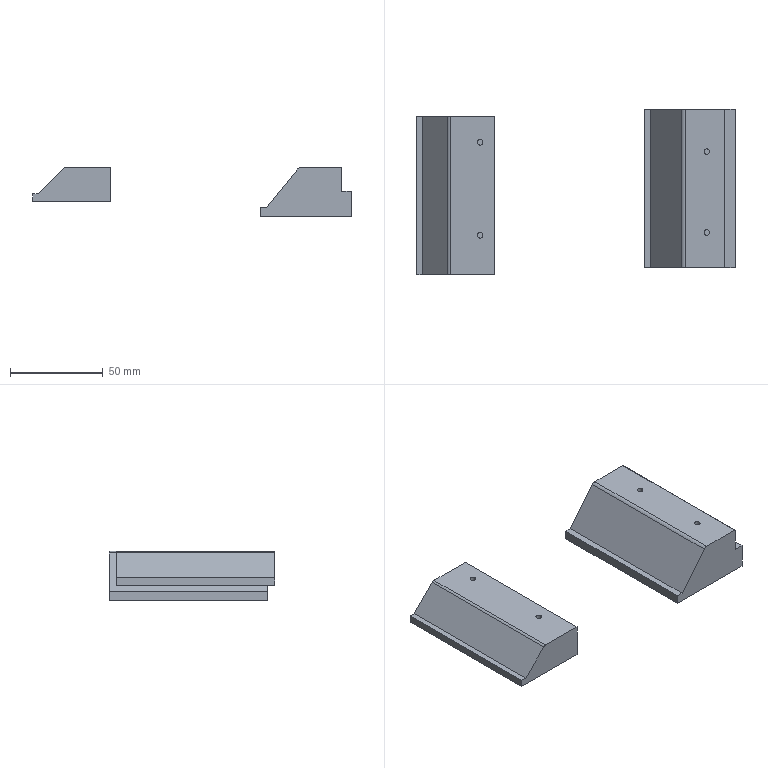NC program | NX | posted with a generic post | part box 171.319 x 88.841 x 26.598 mm
Lines 1 to 928 of 2519:
N10 G17 G21 G94 G90
(FLOOR_WALL_COPY , TOOL : D80)
N12 T19 M6
N14 G54
N16 G17 G0 G90 X91.5 Y0. S6500 M3
N18 G43 Z30. H19
N20 Z3.
N22 G94 G1 Z0. F1500.
N24 X86.5
N26 X-86.5
N28 X-91.5
N30 Z3.
N32 G0 Z30.
N34 M5
(ADAPTIVE_MILLING , TOOL : D10)
N36 T15 M6
N38 G54
N40 G17 G0 G90 X0.049 Y-32.696 S9500 M3
N42 G43 Z30. H15
N44 Z-15.302
N46 G94 G1 Z-18.302 F1000.
N48 X0.579 Y-31.339 F3000.
N50 G3 X0.049 Y-30.049 R1.015
N52 X-3.11 Y-29.406 R9.424
N54 X-14.606 Y-29.21 R185.073
N56 G1 X-20.006 Y-29.208
N58 X-43.706 Y-29.207
N60 X-43.906 Y-29.205
N62 X-44.006 Y-29.201
N64 X-44.106 Y-29.195
N66 X-44.206 Y-29.187
N68 G2 X-48.539 Y-26.275 R6.033
N70 X-50.327 Y-20.706 R13.143
N72 X-50.675 Y-12.117 R79.626
N74 G1 X-50.681 Y-10.617
N76 X-50.686 Y-8.517
N78 X-50.689 Y-4.917
N80 X-50.69 Y8.783
N82 Y22.283
N84 X-50.689 Y22.383
N86 G2 X-48.028 Y26.859 R5.823
N88 X-42.511 Y28.786 R12.484
N90 X-34.025 Y29.173 R71.151
N92 G1 X-32.625 Y29.18
N94 X-30.725 Y29.185
N96 X-27.725 Y29.188
N98 X-20.025 Y29.19
N100 X43.775
N102 X43.875 Y29.189
N104 G2 X48.354 Y26.533 R5.826
N106 X50.283 Y21.017 R12.389
N108 X50.675 Y12.031 R75.333
N110 G1 X50.682 Y10.532
N112 X50.687 Y8.332
N114 X50.689 Y4.632
N116 X50.69 Y-10.868
N118 Y-22.268
N120 Y-22.368
N122 G2 X48.201 Y-26.732 R5.739
N124 X42.821 Y-28.739 R11.862
N126 X34.639 Y-29.167 R61.998
N128 G1 X33.439 Y-29.176
N130 X31.839 Y-29.182
N132 X29.639 Y-29.187
N134 X25.639 Y-29.189
N136 X3.439 Y-29.19
N138 X3.239 Y-29.188
N140 G2 X-2.538 Y-28.69 R147.004
N142 G3 X-15.232 Y-28.421 R195.936
N144 G1 X-18.532 Y-28.418
N146 X-26.232 Y-28.416
N148 X-41.032
N150 X-41.232 Y-28.412
N152 X-41.432 Y-28.404
N154 X-41.532 Y-28.399
N156 G2 X-47.575 Y-24.475 R7.686
N158 X-49.495 Y-18.109 R15.826
N160 X-49.867 Y-8.321 R95.592
N162 G1 X-49.873 Y-6.621
N164 X-49.878 Y-4.221
N166 X-49.881 Y-0.021
N168 X-49.882 Y19.479
N170 X-49.88 Y19.679
N172 X-49.874 Y19.879
N174 G2 X-46.163 Y25.942 R7.587
N176 X-40.032 Y27.941 R15.014
N178 X-30.948 Y28.36 R78.1
N180 G1 X-29.548 Y28.368
N182 X-27.748 Y28.374
N184 X-25.148 Y28.379
N186 X-20.248 Y28.381
N188 X40.952
N190 X41.152 Y28.38
N192 G2 X47.481 Y24.6 R7.579
N194 X49.472 Y18.259 R15.403
N196 X49.867 Y8.172 R92.32
N198 G1 X49.873 Y6.472
N200 X49.878 Y3.972
N202 X49.881 Y-0.428
N204 X49.882 Y-19.528
N206 X49.881 Y-19.628
N208 X49.876 Y-19.827
N210 G2 X46.122 Y-25.967 R7.584
N212 X39.785 Y-27.971 R15.294
N214 X30.498 Y-28.362 R85.233
N216 G1 X28.898 Y-28.37
N218 X26.898 Y-28.376
N220 X23.798 Y-28.38
N222 X16.498 Y-28.381
N224 X5.499
N226 X5.099 Y-28.378
N228 G2 X-3.085 Y-27.873 R210.409
N230 G3 X-18.281 Y-27.628 R312.582
N232 G1 X-22.781 Y-27.625
N234 X-38.381 Y-27.624
N236 X-38.681 Y-27.622
N238 X-38.881 Y-27.619
N240 X-39.081 Y-27.615
N242 X-39.181 Y-27.612
N244 G2 X-44.37 Y-25.752 R8.639
N246 X-46.184 Y-24.587 R5.143
N248 X-47.547 Y-22.113 R6.288
N250 X-48.887 Y-13.949 R30.259
N252 X-49.072 Y2.949 R395.598
N254 G1 X-49.073 Y17.149
N256 X-49.072 Y17.349
N258 X-49.068 Y17.548
N260 X-49.061 Y17.748
N262 X-49.053 Y17.948
N264 X-49.047 Y18.048
N266 G2 X-47.297 Y22.761 R8.54
N268 X-46.087 Y24.683 R5.255
N270 X-43.613 Y26.047 R6.288
N272 X-35.449 Y27.386 R30.365
N274 X-19.151 Y27.572 R379.1
N276 G1 X-5.251 Y27.573
N278 X38.749
N280 X38.949 Y27.57
N282 X39.149 Y27.565
N284 X39.348 Y27.557
N286 G2 X44.262 Y25.797 R8.56
N288 X46.184 Y24.587 R5.254
N290 X47.547 Y22.113 R6.288
N292 X48.885 Y13.948 R30.595
N294 X49.071 Y-0.849 R335.398
N296 G1 X49.073 Y-8.449
N298 Y-17.249
N300 X49.07 Y-17.449
N302 X49.065 Y-17.649
N304 X49.057 Y-17.849
N306 X49.052 Y-17.949
N308 G2 X47.297 Y-22.761 R8.526
N310 X46.087 Y-24.683 R5.256
N312 X43.613 Y-26.047 R6.288
N314 X35.549 Y-27.382 R30.227
N316 X22.751 Y-27.569 R288.936
N318 X5.052 Y-27.536 R956.102
N320 G1 X4.452 Y-27.515
N322 X3.853 Y-27.49
N324 X3.253 Y-27.462
N326 X2.654 Y-27.429
N328 X1.856 Y-27.38
N330 X0.259 Y-27.277
N332 X-0.639 Y-27.224
N334 X-1.937 Y-27.15
N336 X-3.036 Y-27.091
N338 X-3.735 Y-27.057
N340 X-4.235 Y-27.037
N342 G3 X-23.332 Y-26.835 R538.305
N344 G2 X-37.632 Y-26.796 R810.798
N346 X-40.964 Y-26.15 R15.112
N348 X-43.897 Y-25.948 R12.271
N350 G1 X-44.451 Y-25.719
N352 X-44.796 Y-25.58
N354 X-45.13 Y-25.418
N356 G2 X-47.448 Y-22.396 R5.486
N358 X-47.69 Y-19.467 R17.022
N360 X-48.252 Y-3.482 R186.167
N362 G1 X-48.258 Y-1.182
N364 X-48.262 Y2.218
N366 X-48.264 Y8.918
N368 Y15.118
N370 X-48.263 Y15.318
N372 X-48.26 Y15.518
N374 G2 X-47.65 Y19.339 R14.578
N376 X-47.448 Y22.396 R12.938
N378 G1 X-47.295 Y22.766
N380 G3 X-49.411 Y23.198 R-1.1
N382 G1 X-49.85 Y-20.355
N384 G3 X-48.759 Y-21.464 R1.1
N386 X-47.65 Y-20.366 R1.1
N388 G1 Y19.434
N390 G2 X-47.448 Y22.396 R12.58
N392 X-45.011 Y25.486 R5.459
N394 G1 X-43.897 Y25.948
N396 G2 X-40.967 Y26.19 R17.021
N398 X-24.981 Y26.751 R185.822
N400 G1 X-22.781 Y26.757
N402 X-19.481 Y26.762
N404 X-13.581 Y26.764
N406 X36.619
N408 X36.819 Y26.762
N410 X37.018 Y26.759
N412 G2 X40.841 Y26.15 R14.616
N414 X43.897 Y25.948 R12.924
N416 G1 X44.266 Y25.795
N418 G3 X44.693 Y27.911 R-1.1
N420 G1 X-41.86 Y28.35
N422 G3 X-42.964 Y27.254 R1.1
N424 X-41.866 Y26.15 R1.1
N426 G1 X40.934
N428 G2 X43.897 Y25.948 R12.58
N430 X46.986 Y23.511 R5.459
N432 G1 X47.448 Y22.396
N434 G2 X47.679 Y19.666 R14.737
N436 X48.255 Y2.281 R199.943
N438 G1 X48.26 Y-0.319
N440 X48.263 Y-4.519
N442 X48.264 Y-15.019
N444 X48.263 Y-15.319
N446 X48.26 Y-15.519
N448 X48.255 Y-15.718
N450 G2 X47.65 Y-19.34 R14.715
N452 X47.448 Y-22.396 R12.93
N454 G1 X47.295 Y-22.766
N456 G3 X49.411 Y-23.198 R-1.1
N458 G1 X49.85 Y20.355
N460 G3 X48.759 Y21.464 R1.1
N462 X47.65 Y20.366 R1.1
N464 G1 Y-19.434
N466 G2 X47.448 Y-22.396 R12.58
N468 X45.011 Y-25.486 R5.459
N470 G1 X43.897 Y-25.948
N472 G2 X40.967 Y-26.19 R17.021
N474 X24.782 Y-26.752 R186.361
N476 X5.082 Y-26.699 R835.083
N478 G3 X-7.755 Y-26.15 R639.752
N480 G1 X-41.055
N482 G3 X-42.153 Y-27.252 R1.1
N484 X-41.055 Y-28.35 R1.1
N486 G1 X41.866
N488 G3 X42.964 Y-27.248 R1.1
N490 X41.866 Y-26.15 R1.1
N492 G1 X-7.834
N494 G3 X-8.832 Y-27.001 R1.016
N496 G1 X-9.082 Y-28.572
N498 Z-15.302
N500 G0 Z30.
N502 X50.031 Y-18.162
N504 Z-10.486
N506 G1 Z-13.486 F1000.
N508 X49.292 Y-17.946 F3000.
N510 X48.547 Y-17.752
N512 G3 X47.452 Y-18.495 R1.016
N514 G2 X45.984 Y-21.956 R6.556
N516 X41.078 Y-24.678 R9.318
N518 X34.326 Y-25.371 R32.522
N520 X20.727 Y-25.44 R724.644
N522 G1 X-39.873 Y-25.441
N524 X-40.073 Y-25.437
N526 X-40.273 Y-25.429
N528 X-40.373 Y-25.422
N530 G2 X-44.753 Y-22.45 R5.792
N532 G3 X-45.418 Y-21.357 R5.86
N534 G2 X-47.577 Y-17.693 R4.949
N536 G3 X-49.483 Y-17.412 R1.001
N538 G1 X-49.569 Y-17.734 Z-13.469
N540 X-49.611 Y-18.065 Z-13.452
N542 X-49.785 Y-19.386 Z-13.386
N544 X-49.898 Y-20.216
N546 X-49.995 Y-21.048
N548 G3 X-49.827 Y-21.59 R1.053
N550 G1 X-48.847 Y-23.037
N552 G3 X-47.505 Y-24.5 R10.089
N554 G1 X-44.694 Y-26.992
N556 G3 X-42.548 Y-28.08 R4.811
N558 X-40.089 Y-28.362 R12.881
N560 G1 X-25.715 Y-28.562
N562 X-13.22 Y-28.683
N564 X29.282 Y-28.993
N566 G3 X40.432 Y-27.976 R57.483
N568 G1 X41.987 Y-27.682
N570 X43.538 Y-27.368
N572 G3 X47.827 Y-24.665 R8.195
N574 G1 X49.697 Y-22.41
N576 G3 X49.909 Y-21.582 R1.016
N578 G1 X49.587 Y-19.917
N580 X49.459 Y-19.235 Z-13.42
N582 X49.313 Y-18.557 Z-13.455
N584 G3 X48.948 Y-18.077 Z-13.486 R1.046
N586 X47.447 Y-18.513 R1.003
N588 G2 X45.131 Y-21.56 R5.566
N590 X37.949 Y-24.134 R16.415
N592 X28.768 Y-24.605 R73.474
N594 G1 X27.468 Y-24.615
N596 X25.968 Y-24.622
N598 X23.868 Y-24.627
N600 X20.568 Y-24.631
N602 X12.468 Y-24.632
N604 X-37.232
N606 G2 X-41.953 Y-22.956 R7.857
N608 G3 X-43.08 Y-22.245 R4.016
N610 G2 X-45.456 Y-21.328 R4.637
N612 G3 X-47.012 Y-22.452 R1.001
N614 G1 X-46.855 Y-22.733 Z-13.47
N616 X-46.651 Y-22.981 Z-13.453
N618 X-45.782 Y-24.021 Z-13.386
N620 X-44.517 Y-25.52
N622 X-44.291 Y-25.674
N624 X-42.723 Y-26.445
N626 G3 X-40.227 Y-27.196 R12.103
N628 X-36.527 Y-27.61 R17.873
N630 G1 X-7.776 Y-27.757
N632 X-0.589 Y-27.781
N634 X6.598 Y-27.776
N636 X13.786 Y-27.744
N638 X20.973 Y-27.685
N640 X32.849 Y-27.564
N642 G3 X39.047 Y-26.949 R36.726
N644 G1 X40.883 Y-26.584
N646 X42.708 Y-26.163
N648 X46.088 Y-25.315
N650 G3 X46.799 Y-24.643 R1.014
N652 G1 X47.297 Y-23.054
N654 X47.505 Y-22.404 Z-13.42
N656 X47.692 Y-21.748 Z-13.454
N658 G3 X47.585 Y-21.133 Z-13.486 R1.043
N660 X46.088 Y-20.815 R1.004
N662 G1 X45.131 Y-21.56
N664 G2 X42.689 Y-22.35 R6.963
N666 X30.293 Y-23.746 R56.102
N668 X15.594 Y-23.823 R755.81
N670 G1 X-6.906 Y-23.824
N672 X-34.806
N674 X-35.106 Y-23.821
N676 X-35.306 Y-23.816
N678 X-35.506 Y-23.809
N680 G2 X-40.49 Y-22.447 R13.721
N682 G1 X-40.583 Y-22.41
N684 X-40.677 Y-22.375
N686 X-40.773 Y-22.349
N688 X-40.871 Y-22.331
N690 X-40.931 Y-22.325
N692 G2 X-43.13 Y-22.238 R12.199
N694 G3 X-43.279 Y-24.428 R-1.1
N696 G1 X43.828 Y-24.344
N698 G3 X43.669 Y-22.155 R-1.1
N700 G2 X40.762 Y-22.325 R12.892
N702 X32.479 Y-22.844 R767.671
N704 X13.681 Y-23.014 R575.765
N706 G1 X-4.719 Y-23.015
N708 X-32.719
N710 X-33.019 Y-23.013
N712 X-33.219 Y-23.01
N714 X-33.419 Y-23.006
N716 X-33.719 Y-22.995
N718 G2 X-37.84 Y-22.325 R20.053
N720 G1 X-40.94
N722 G3 X-42.038 Y-23.426 R1.1
N724 X-40.94 Y-24.525 R1.1
N726 G1 X40.762
N728 G3 X41.86 Y-23.423 R1.1
N730 X40.762 Y-22.325 R1.1
N732 G1 X-37.938
N734 G3 X-38.935 Y-23.497 R1.014
N736 G1 X-38.72 Y-24.815
N738 Z-10.486
N740 G0 Z30.
N742 X50.15 Y-15.545
N744 Z-9.522
N746 G1 Z-12.522 F1000.
N748 X48.445 Y-15.788 F3000.
N750 G3 X47.585 Y-16.662 R1.017
N752 G2 X46.929 Y-18.8 R5.231
N754 X43.771 Y-21.186 R5.494
N756 X40.065 Y-21.424 R21.422
N758 G1 X39.065 Y-21.437
N760 X38.065 Y-21.447
N762 X36.665 Y-21.454
N764 X34.765 Y-21.46
N766 X31.865 Y-21.464
N768 X25.065 Y-21.465
N770 X-39.735
N772 X-39.935 Y-21.464
N774 X-40.035 Y-21.461
N776 X-40.135 Y-21.456
N778 G3 X-42.536 Y-21.356 R13.621
N780 G2 X-46.099 Y-19.865 R5.576
N782 X-47.49 Y-17.424 R5.74
N784 G1 X-47.59 Y-16.631
N786 G3 X-49.449 Y-16.258 R1.001
N788 G1 X-49.56 Y-16.555 Z-12.507
N790 X-49.618 Y-16.867 Z-12.491
N792 X-49.859 Y-18.21 Z-12.422
N794 X-50.008 Y-19.005
N796 X-50.132 Y-19.804
N798 G3 X-49.84 Y-20.528 R1.026
N800 G1 X-48.813 Y-21.561
N802 X-47.769 Y-22.578
N804 G3 X-45.555 Y-23.78 R6.079
N806 X-43.616 Y-24.16 R9.286
N808 X-37.387 Y-24.471 R69.76
N810 G1 X39.401 Y-24.536
N812 X39.631 Y-24.481
N814 X41.825 Y-23.665
N816 X42.394 Y-23.458 Z-12.453
N818 X42.955 Y-23.232 Z-12.483
N820 G3 X43.428 Y-22.626 Z-12.522 R1.027
N822 X42.464 Y-21.361 R1.003
N824 G1 X-40.936
N826 G3 X-41.937 Y-22.239 R1.015
N828 G1 X-42.151 Y-23.861
N830 Z-9.522
N832 G0 Z30.
N834 X50.15 Y-14.577
N836 Z-8.559
N838 G1 Z-11.559 F1000.
N840 X48.445 Y-14.821 F3000.
N842 G3 X47.586 Y-15.695 R1.017
N844 G2 X46.929 Y-17.837 R5.235
N846 X43.771 Y-20.223 R5.494
N848 X40.065 Y-20.461 R21.422
N850 G1 X39.065 Y-20.474
N852 X38.065 Y-20.483
N854 X36.665 Y-20.491
N856 X34.765 Y-20.497
N858 X31.865 Y-20.5
N860 X25.065 Y-20.502
N862 X-39.735
N864 X-39.935 Y-20.501
N866 X-40.035 Y-20.498
N868 X-40.135 Y-20.493
N870 G3 X-42.536 Y-20.393 R13.617
N872 G2 X-46.099 Y-18.901 R5.576
N874 X-47.49 Y-16.461 R5.74
N876 G1 X-47.59 Y-15.667
N878 G3 X-49.449 Y-15.295 R1.001
N880 G1 X-49.56 Y-15.592 Z-11.543
N882 X-49.618 Y-15.903 Z-11.527
N884 X-49.859 Y-17.246 Z-11.459
N886 X-50.008 Y-18.041
N888 X-50.132 Y-18.84
N890 G3 X-49.84 Y-19.565 R1.026
N892 G1 X-48.813 Y-20.598
N894 X-47.769 Y-21.614
N896 G3 X-45.555 Y-22.817 R6.079
N898 X-43.616 Y-23.197 R9.286
N900 X-37.387 Y-23.508 R69.76
N902 G1 X39.401 Y-23.573
N904 X39.631 Y-23.517
N906 X41.825 Y-22.702
N908 X42.394 Y-22.494 Z-11.489
N910 X42.955 Y-22.269 Z-11.52
N912 G3 X43.428 Y-21.663 Z-11.559 R1.027
N914 X42.464 Y-20.398 R1.003
N916 G1 X-40.936
N918 G3 X-41.937 Y-21.276 R1.015
N920 G1 X-42.151 Y-22.897
N922 Z-8.559
N924 G0 Z30.
N926 X50.15 Y-13.613
N928 Z-7.596
N930 G1 Z-10.596 F1000.
N932 X48.445 Y-13.857 F3000.
N934 G3 X47.586 Y-14.731 R1.017
N936 G2 X46.929 Y-16.873 R5.235
N938 X43.771 Y-19.26 R5.494
N940 X40.065 Y-19.498 R21.423
N942 G1 X39.065 Y-19.511
N944 X38.065 Y-19.52
N946 X36.665 Y-19.528
N948 X34.765 Y-19.533
N950 X31.865 Y-19.537
N952 X25.165 Y-19.539
N954 X-39.735
N956 X-39.935 Y-19.537
N958 X-40.035 Y-19.535
N960 X-40.135 Y-19.529
N962 G3 X-42.536 Y-19.43 R13.617
N964 G2 X-46.099 Y-17.938 R5.575
N966 X-47.49 Y-15.498 R5.74
N968 G1 X-47.59 Y-14.704
N970 G3 X-49.449 Y-14.332 R1.001
N972 G1 X-49.56 Y-14.628 Z-10.58
N974 X-49.618 Y-14.94 Z-10.564
N976 X-49.859 Y-16.283 Z-10.496
N978 X-50.008 Y-17.078
N980 X-50.132 Y-17.877
N982 G3 X-49.84 Y-18.601 R1.026
N984 G1 X-48.813 Y-19.634
N986 X-47.769 Y-20.651
N988 G3 X-45.555 Y-21.853 R6.079
N990 X-43.616 Y-22.233 R9.286
N992 X-37.387 Y-22.544 R69.76
N994 G1 X39.401 Y-22.61
N996 X39.631 Y-22.554
N998 X41.825 Y-21.739
N1000 X42.394 Y-21.531 Z-10.526
N1002 X42.955 Y-21.306 Z-10.556
N1004 G3 X43.428 Y-20.7 Z-10.596 R1.027
N1006 X42.464 Y-19.435 R1.003
N1008 G1 X-40.936
N1010 G3 X-41.937 Y-20.313 R1.015
N1012 G1 X-42.151 Y-21.934
N1014 Z-7.596
N1016 G0 Z30.
N1018 X50.15 Y-12.65
N1020 Z-6.633
N1022 G1 Z-9.633 F1000.
N1024 X48.445 Y-12.894 F3000.
N1026 G3 X47.586 Y-13.768 R1.017
N1028 G2 X46.929 Y-15.91 R5.235
N1030 X43.771 Y-18.296 R5.494
N1032 X40.065 Y-18.535 R21.423
N1034 G1 X39.065 Y-18.548
N1036 X38.065 Y-18.557
N1038 X36.665 Y-18.564
N1040 X34.765 Y-18.57
N1042 X31.865 Y-18.574
N1044 X25.165 Y-18.575
N1046 X-39.735 Y-18.576
N1048 X-39.935 Y-18.574
N1050 X-40.035 Y-18.571
N1052 X-40.135 Y-18.566
N1054 G3 X-42.536 Y-18.467 R13.617
N1056 G2 X-46.099 Y-16.975 R5.575
N1058 X-47.49 Y-14.535 R5.74
N1060 G1 X-47.59 Y-13.741
N1062 G3 X-49.449 Y-13.368 R1.001
N1064 G1 X-49.56 Y-13.665 Z-9.617
N1066 X-49.618 Y-13.977 Z-9.601
N1068 X-49.859 Y-15.32 Z-9.533
N1070 X-50.008 Y-16.115
N1072 X-50.132 Y-16.914
N1074 G3 X-49.84 Y-17.638 R1.026
N1076 G1 X-48.813 Y-18.671
N1078 X-47.769 Y-19.688
N1080 G3 X-45.555 Y-20.89 R6.079
N1082 X-43.616 Y-21.27 R9.286
N1084 X-37.387 Y-21.581 R69.76
N1086 G1 X39.401 Y-21.646
N1088 X39.631 Y-21.591
N1090 X41.825 Y-20.776
N1092 X42.394 Y-20.568 Z-9.563
N1094 X42.955 Y-20.342 Z-9.593
N1096 G3 X43.428 Y-19.736 Z-9.633 R1.027
N1098 X42.464 Y-18.471 R1.003
N1100 G1 X-40.936
N1102 G3 X-41.937 Y-19.349 R1.015
N1104 G1 X-42.151 Y-20.971
N1106 Z-6.633
N1108 G0 Z30.
N1110 X50.15 Y-11.687
N1112 Z-5.669
N1114 G1 Z-8.669 F1000.
N1116 X48.445 Y-11.931 F3000.
N1118 G3 X47.586 Y-12.805 R1.017
N1120 G2 X46.929 Y-14.947 R5.235
N1122 X43.771 Y-17.333 R5.494
N1124 X40.065 Y-17.571 R21.423
N1126 G1 X39.065 Y-17.584
N1128 X38.065 Y-17.593
N1130 X36.665 Y-17.601
N1132 X34.765 Y-17.607
N1134 X31.865 Y-17.611
N1136 X25.065 Y-17.612
N1138 X-39.735
N1140 X-39.935 Y-17.611
N1142 X-40.035 Y-17.608
N1144 X-40.135 Y-17.603
N1146 G3 X-42.536 Y-17.503 R13.617
N1148 G2 X-46.099 Y-16.012 R5.575
N1150 X-47.49 Y-13.571 R5.74
N1152 G1 X-47.59 Y-12.778
N1154 G3 X-49.449 Y-12.405 R1.001
N1156 G1 X-49.56 Y-12.702 Z-8.654
N1158 X-49.618 Y-13.013 Z-8.638
N1160 X-49.859 Y-14.357 Z-8.569
N1162 X-50.008 Y-15.151
N1164 X-50.132 Y-15.95
N1166 G3 X-49.84 Y-16.675 R1.026
N1168 G1 X-48.813 Y-17.708
N1170 X-47.769 Y-18.724
N1172 G3 X-45.555 Y-19.927 R6.079
N1174 X-43.616 Y-20.307 R9.286
N1176 X-37.387 Y-20.618 R69.76
N1178 G1 X39.401 Y-20.683
N1180 X39.631 Y-20.628
N1182 X41.825 Y-19.812
N1184 X42.394 Y-19.604 Z-8.6
N1186 X42.955 Y-19.379 Z-8.63
N1188 G3 X43.428 Y-18.773 Z-8.669 R1.027
N1190 X42.464 Y-17.508 R1.003
N1192 G1 X-40.936
N1194 G3 X-41.937 Y-18.386 R1.015
N1196 G1 X-42.151 Y-20.007
N1198 Z-5.669
N1200 G0 Z30.
N1202 X50.15 Y-10.723
N1204 Z-4.706
N1206 G1 Z-7.706 F1000.
N1208 X48.445 Y-10.967 F3000.
N1210 G3 X47.586 Y-11.841 R1.017
N1212 G2 X46.929 Y-13.983 R5.235
N1214 X43.771 Y-16.37 R5.494
N1216 X40.065 Y-16.608 R21.423
N1218 G1 X39.065 Y-16.621
N1220 X38.065 Y-16.63
N1222 X36.665 Y-16.638
N1224 X34.765 Y-16.644
N1226 X31.865 Y-16.647
N1228 X25.165 Y-16.649
N1230 X-39.735
N1232 X-39.935 Y-16.648
N1234 X-40.035 Y-16.645
N1236 X-40.135 Y-16.64
N1238 G3 X-42.536 Y-16.54 R13.617
N1240 G2 X-46.099 Y-15.048 R5.575
N1242 X-47.49 Y-12.608 R5.74
N1244 G1 X-47.59 Y-11.814
N1246 G3 X-49.449 Y-11.442 R1.001
N1248 G1 X-49.56 Y-11.739 Z-7.69
N1250 X-49.618 Y-12.05 Z-7.674
N1252 X-49.859 Y-13.393 Z-7.606
N1254 X-50.008 Y-14.188
N1256 X-50.132 Y-14.987
N1258 G3 X-49.84 Y-15.711 R1.026
N1260 G1 X-48.813 Y-16.745
N1262 X-47.769 Y-17.761
N1264 G3 X-45.555 Y-18.964 R6.079
N1266 X-43.616 Y-19.344 R9.286
N1268 X-37.387 Y-19.654 R69.76
N1270 G1 X39.401 Y-19.72
N1272 X39.631 Y-19.664
N1274 X41.825 Y-18.849
N1276 X42.394 Y-18.641 Z-7.636
N1278 X42.955 Y-18.416 Z-7.667
N1280 G3 X43.428 Y-17.81 Z-7.706 R1.027
N1282 X42.464 Y-16.545 R1.003
N1284 G1 X-40.936
N1286 G3 X-41.937 Y-17.423 R1.015
N1288 G1 X-42.151 Y-19.044
N1290 Z-4.706
N1292 G0 Z30.
N1294 X50.15 Y-9.76
N1296 Z-3.743
N1298 G1 Z-6.743 F1000.
N1300 X48.445 Y-10.004 F3000.
N1302 G3 X47.586 Y-10.878 R1.017
N1304 G2 X46.929 Y-13.02 R5.235
N1306 X43.771 Y-15.406 R5.494
N1308 X40.065 Y-15.645 R21.423
N1310 G1 X39.065 Y-15.658
N1312 X38.065 Y-15.667
N1314 X36.665 Y-15.675
N1316 X34.765 Y-15.68
N1318 X31.865 Y-15.684
N1320 X25.165 Y-15.686
N1322 X-39.735
N1324 X-39.935 Y-15.684
N1326 X-40.035 Y-15.681
N1328 X-40.135 Y-15.676
N1330 G3 X-42.536 Y-15.577 R13.617
N1332 G2 X-46.099 Y-14.085 R5.575
N1334 X-47.49 Y-11.645 R5.74
N1336 G1 X-47.59 Y-10.851
N1338 G3 X-49.449 Y-10.478 R1.001
N1340 G1 X-49.56 Y-10.775 Z-6.727
N1342 X-49.618 Y-11.087 Z-6.711
N1344 X-49.859 Y-12.43 Z-6.643
N1346 X-50.008 Y-13.225
N1348 X-50.132 Y-14.024
N1350 G3 X-49.84 Y-14.748 R1.026
N1352 G1 X-48.813 Y-15.781
N1354 X-47.769 Y-16.798
N1356 G3 X-45.555 Y-18. R6.079
N1358 X-43.616 Y-18.38 R9.286
N1360 X-37.387 Y-18.691 R69.76
N1362 G1 X39.401 Y-18.757
N1364 X39.631 Y-18.701
N1366 X41.825 Y-17.886
N1368 X42.394 Y-17.678 Z-6.673
N1370 X42.955 Y-17.453 Z-6.703
N1372 G3 X43.428 Y-16.847 Z-6.743 R1.027
N1374 X42.464 Y-15.582 R1.003
N1376 G1 X-40.936
N1378 G3 X-41.937 Y-16.46 R1.015
N1380 G1 X-42.151 Y-18.081
N1382 Z-3.743
N1384 G0 Z30.
N1386 X50.15 Y-8.797
N1388 Z-2.78
N1390 G1 Z-5.78 F1000.
N1392 X48.445 Y-9.041 F3000.
N1394 G3 X47.586 Y-9.915 R1.017
N1396 G2 X46.929 Y-12.057 R5.235
N1398 X43.771 Y-14.443 R5.494
N1400 X40.065 Y-14.681 R21.423
N1402 G1 X39.065 Y-14.694
N1404 X38.065 Y-14.704
N1406 X36.665 Y-14.711
N1408 X34.765 Y-14.717
N1410 X31.865 Y-14.721
N1412 X25.165 Y-14.722
N1414 X-39.735
N1416 X-39.935 Y-14.721
N1418 X-40.035 Y-14.718
N1420 X-40.135 Y-14.713
N1422 G3 X-42.536 Y-14.613 R13.621
N1424 G2 X-46.099 Y-13.122 R5.575
N1426 X-47.49 Y-10.681 R5.74
N1428 G1 X-47.59 Y-9.888
N1430 G3 X-49.449 Y-9.515 R1.001
N1432 G1 X-49.56 Y-9.812 Z-5.764
N1434 X-49.618 Y-10.124 Z-5.748
N1436 X-49.859 Y-11.467 Z-5.68
N1438 X-50.008 Y-12.262
N1440 X-50.132 Y-13.061
N1442 G3 X-49.84 Y-13.785 R1.026
N1444 G1 X-48.813 Y-14.818
N1446 X-47.769 Y-15.835
N1448 G3 X-45.555 Y-17.037 R6.079
N1450 X-43.616 Y-17.417 R9.286
N1452 X-37.387 Y-17.728 R69.76
N1454 G1 X39.401 Y-17.793
N1456 X39.631 Y-17.738
N1458 X41.825 Y-16.922
N1460 X42.394 Y-16.715 Z-5.71
N1462 X42.955 Y-16.489 Z-5.74
N1464 G3 X43.428 Y-15.883 Z-5.78 R1.027
N1466 X42.464 Y-14.618 R1.003
N1468 G1 X-40.936
N1470 G3 X-41.937 Y-15.496 R1.015
N1472 G1 X-42.151 Y-17.118
N1474 Z-2.78
N1476 G0 Z30.
N1478 X50.15 Y-6.883
N1480 Z-0.853
N1482 G1 Z-3.853 F1000.
N1484 X48.445 Y-7.124 F3000.
N1486 G3 X47.585 Y-7.999 R1.017
N1488 G2 X45.67 Y-11.529 R4.877
N1490 X42.626 Y-13. R7.829
N1492 X35.793 Y-13.825 R28.455
N1494 X18.293 Y-13.906 R831.629
N1496 G1 X-39.907 Y-13.9
N1498 X-40.007 Y-13.898
N1500 X-40.106 Y-13.893
N1502 X-40.206 Y-13.887
N1504 X-40.306 Y-13.879
N1506 G2 X-43.121 Y-12.681 R5.606
N1508 G3 X-43.903 Y-12.481 R3.74
N1510 G2 X-46.997 Y-10.012 R5.494
N1512 X-47.577 Y-8.06 R5.251
N1514 G3 X-49.415 Y-7.651 R1.001
N1516 X-49.604 Y-8.289 Z-3.82 R1.691
N1518 G1 X-49.839 Y-9.598 Z-3.753
N1520 X-49.992 Y-10.413
N1522 X-50.12 Y-11.233
N1524 G3 X-49.827 Y-11.957 R1.026
N1526 G1 X-48.117 Y-13.649
N1528 G3 X-45.488 Y-15.426 R11.292
N1530 X-43.111 Y-16.431 R16.001
N1532 X-39.634 Y-16.957 R11.922
N1534 G1 X37.689
N1536 G3 X42.554 Y-16.25 R17.272
N1538 G1 X44.935 Y-15.542
N1540 G3 X45.433 Y-15.205 R1.047
N1542 G1 X46.232 Y-14.199
N1544 X47.475 Y-12.633 Z-3.853
N1546 G3 X46.099 Y-11.195 R1.001
N1548 G1 X45.14 Y-11.94
N1550 X45.022 Y-12.009
N1552 G2 X42.064 Y-12.699 R6.17
N1554 X25.772 Y-13.094 R245.256
N1556 G1 X22.172 Y-13.097
N1558 X13.072
N1560 X-37.128 Y-13.091
N1562 X-37.228
N1564 X-37.428 Y-13.085
N1566 X-37.628 Y-13.076
N1568 G2 X-39.907 Y-12.692 R18.467
N1570 G1 X-42.464
N1572 X-42.536 Y-12.687
N1574 X-43.427 Y-12.564
N1576 G3 X-43.579 Y-14.754 R-1.1
N1578 G1 X42.362 Y-14.892
N1580 G3 X43.462 Y-13.792 R1.1
N1582 X42.364 Y-12.692 R1.1
N1584 G1 X-39.936
N1586 G3 X-40.946 Y-13.714 R1.014
N1588 G1 X-40.928 Y-15.188
N1590 Z-0.853
N1592 G0 Z30.
N1594 X50.15 Y-5.907
N1596 Z0.11
N1598 G1 Z-2.89 F1000.
N1600 X48.445 Y-6.151 F3000.
N1602 G3 X47.586 Y-7.025 R1.017
N1604 G2 X46.929 Y-9.167 R5.235
N1606 X43.771 Y-11.553 R5.494
N1608 X40.065 Y-11.792 R21.422
N1610 G1 X39.065 Y-11.805
N1612 X38.065 Y-11.814
N1614 X36.765 Y-11.821
N1616 X34.965 Y-11.827
N1618 X32.165 Y-11.831
N1620 X25.965 Y-11.832
N1622 X-39.735 Y-11.833
N1624 X-39.935 Y-11.831
N1626 X-40.035 Y-11.828
N1628 X-40.135 Y-11.823
N1630 G3 X-42.536 Y-11.724 R13.61
N1632 G2 X-46.099 Y-10.232 R5.576
N1634 X-47.49 Y-7.792 R5.74
N1636 G1 X-47.59 Y-6.998
N1638 G3 X-49.449 Y-6.625 R1.001
N1640 G1 X-49.56 Y-6.922 Z-2.874
N1642 X-49.618 Y-7.234 Z-2.858
N1644 X-49.859 Y-8.577 Z-2.79
N1646 X-50.008 Y-9.372
N1648 X-50.132 Y-10.171
N1650 G3 X-49.84 Y-10.895 R1.026
N1652 G1 X-48.813 Y-11.928
N1654 X-47.769 Y-12.945
N1656 G3 X-45.555 Y-14.147 R6.079
N1658 X-43.616 Y-14.527 R9.286
N1660 X-37.387 Y-14.838 R69.76
N1662 G1 X39.401 Y-14.903
N1664 X39.631 Y-14.848
N1666 X41.825 Y-14.033
N1668 X42.394 Y-13.825 Z-2.82
N1670 X42.955 Y-13.599 Z-2.85
N1672 G3 X43.428 Y-12.993 Z-2.89 R1.027
N1674 X42.464 Y-11.728 R1.003
N1676 G1 X-40.936
N1678 G3 X-41.937 Y-12.607 R1.015
N1680 G1 X-42.151 Y-14.228
N1682 Z0.11
N1684 G0 Z30.
N1686 X50.15 Y-4.944
N1688 Z1.073
N1690 G1 Z-1.927 F1000.
N1692 X48.445 Y-5.188 F3000.
N1694 G3 X47.586 Y-6.062 R1.017
N1696 G2 X46.929 Y-8.204 R5.235
N1698 X43.771 Y-10.59 R5.494
N1700 X40.065 Y-10.828 R21.422
N1702 G1 X39.065 Y-10.841
N1704 X38.065 Y-10.85
N1706 X36.765 Y-10.858
N1708 X34.965 Y-10.863
N1710 X32.165 Y-10.867
N1712 X25.965 Y-10.869
N1714 X-39.735
N1716 X-39.935 Y-10.868
N1718 X-40.035 Y-10.865
N1720 X-40.135 Y-10.86
N1722 G3 X-42.536 Y-10.76 R13.621
N1724 G2 X-46.099 Y-9.269 R5.576
N1726 X-47.49 Y-6.828 R5.74
N1728 G1 X-47.59 Y-6.035
N1730 G3 X-49.449 Y-5.662 R1.001
N1732 G1 X-49.56 Y-5.959 Z-1.911
N1734 X-49.618 Y-6.27 Z-1.895
N1736 X-49.859 Y-7.614 Z-1.827
N1738 X-50.008 Y-8.408
N1740 X-50.132 Y-9.207
N1742 G3 X-49.84 Y-9.932 R1.026
N1744 G1 X-48.813 Y-10.965
N1746 X-47.769 Y-11.981
N1748 G3 X-45.555 Y-13.184 R6.079
N1750 X-43.616 Y-13.564 R9.286
N1752 X-37.387 Y-13.875 R69.76
N1754 G1 X39.401 Y-13.94
N1756 X39.631 Y-13.885
N1758 X41.825 Y-13.069
N1760 X42.394 Y-12.861 Z-1.857
N1762 X42.955 Y-12.636 Z-1.887
N1764 G3 X43.428 Y-12.03 Z-1.927 R1.027
N1766 X42.464 Y-10.765 R1.003
N1768 G1 X-40.936
N1770 G3 X-41.937 Y-11.643 R1.015
N1772 G1 X-42.151 Y-13.264
N1774 Z1.073
N1776 G0 Z30.
N1778 M5
(ZLEVEL_PROFILE_COPY_1_COPY_COPY_1 , TOOL : D10JING)
N1780 T14 M6
N1782 G54
N1784 G17 G0 G90 X44.122 Y-27.809 S9500 M3
N1786 G43 Z30. H14
N1788 Z-17.302
N1790 G94 G1 Z-18.302 F1000.
N1792 X43.366 Y-26.5
N1794 G3 X42.5 Y-26. R1.
N1796 G1 X-42.5 F1200.
N1798 G2 X-47.5 Y-21. R5.
N1800 G1 Y21.
N1802 G2 X-42.5 Y26. R5.
N1804 G1 X42.5
N1806 G2 X47.5 Y21. R5.
N1808 G1 Y-21.
N1810 G2 X42.5 Y-26. R5.
N1812 G3 X41.634 Y-26.5 R1.
N1814 G1 X40.768 Y-28.
N1816 Z-17.302
N1818 G0 Z30.
(FLOOR_WALL_1 , TOOL : D10JING)
N1820 X50.5 Y-22.929
N1822 Z-11.302
N1824 G1 Z-14.302 F1250.
N1826 X47.5
N1828 X-47.5
N1830 X-50.5
N1832 Z-11.302
N1834 G0 Z30.
N1836 M5